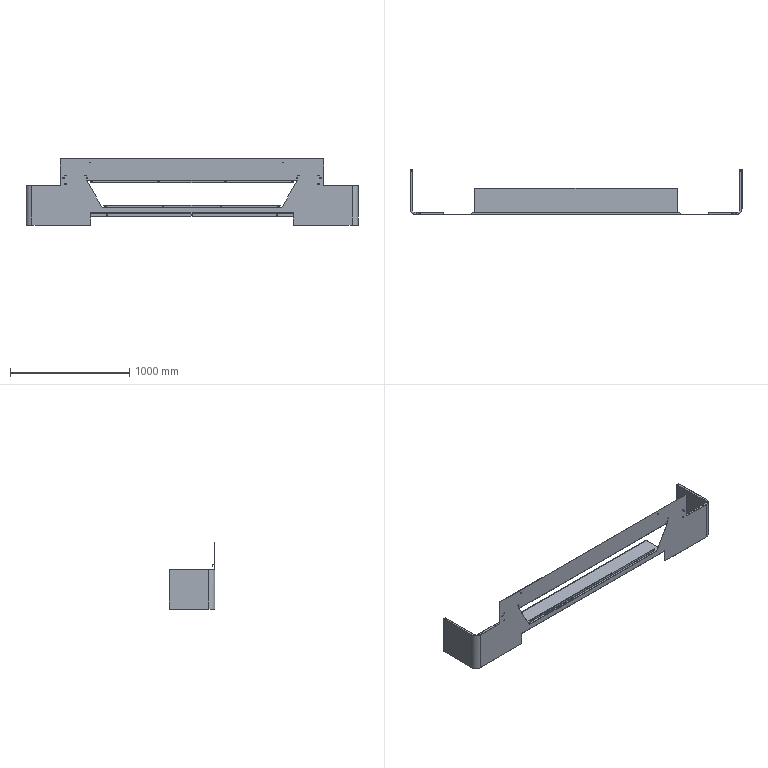Part | SolidWorks | features ICE 20, EdgeFlange 8, SMBaseFlange 5, LPattern 3, MirrorPattern 2, FlatPattern 1, SheetMetal 1 | 1 solid | 304 faces | box 2780 x 380 x 555 mm | volume 2537255 mm3 | plane 217 | cylinder 87 | commonest cylinder face diameters 6 x50 1 x12 4 x12 7 x6 96 x3 97 x2